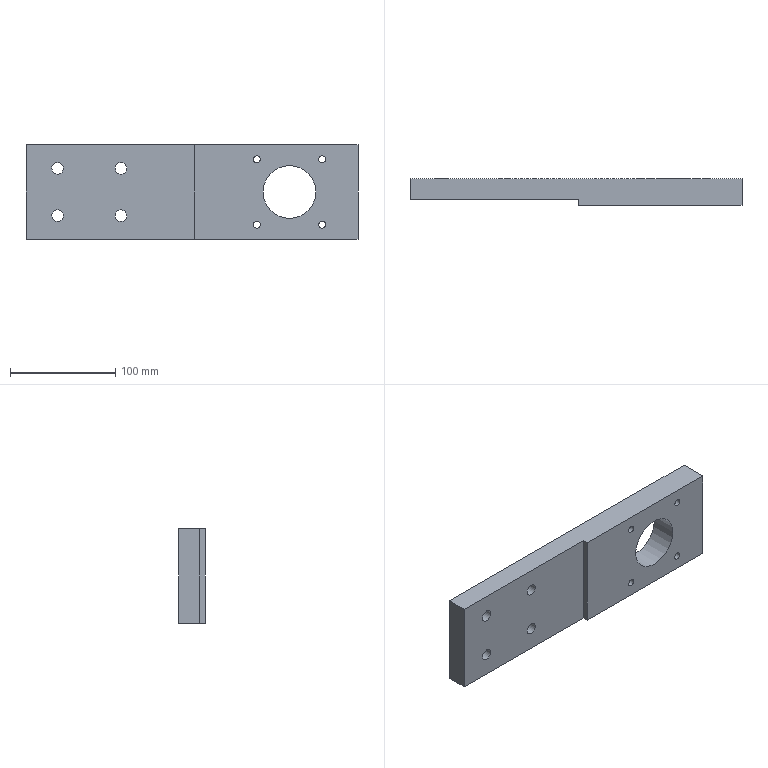Part | STEP file | SN10_002_002_PLACA | 1 solid | 17 faces | box 315 x 25 x 90 mm | volume 576590 mm3 | cylinder 9 | plane 8 | commonest cylinder face diameters 6.647 x4 11 x4 50 x1
STEP:
#1=CARTESIAN_POINT('',(0.,0.,0.));
#2=DIRECTION('',(0.,0.,1.));
#3=DIRECTION('',(1.,0.,0.));
#4=AXIS2_PLACEMENT_3D('',#1,#2,#3);
#5=CARTESIAN_POINT('',(5971.917,200.,32.593));
#6=VERTEX_POINT('',#5);
#7=CARTESIAN_POINT('',(5969.,200.,31.));
#8=DIRECTION('',(0.,-1.,0.));
#9=DIRECTION('',(1.,0.,0.));
#10=AXIS2_PLACEMENT_3D('',#7,#8,#9);
#11=CIRCLE('',#10,3.324);
#12=CARTESIAN_POINT('',(5969.,199.9,31.));
#13=DIRECTION('',(0.,-1.,0.));
#14=DIRECTION('',(0.8776,0.,0.4794));
#15=AXIS2_PLACEMENT_3D('',#12,#13,#14);
#16=CYLINDRICAL_SURFACE('',#15,3.324);
#17=CARTESIAN_POINT('',(-0.5,-0.1));
#18=DIRECTION('',(1.,0.));
#19=VECTOR('',#18,1.);
#20=LINE('',#17,#19);
#21=(GEOMETRIC_REPRESENTATION_CONTEXT(2)PARAMETRIC_REPRESENTATION_CONTEXT()REPRESENTATION_CONTEXT('',''));
#22=DEFINITIONAL_REPRESENTATION('',(#20),#21);
#23=PCURVE('',#16,#22);
#24=CARTESIAN_POINT('',(6065.,200.,45.));
#25=DIRECTION('',(0.,-1.,0.));
#26=DIRECTION('',(0.,0.,-1.));
#27=AXIS2_PLACEMENT_3D('',#24,#25,#26);
#28=PLANE('',#27);
#29=CARTESIAN_POINT('',(14.,-96.));
#30=DIRECTION('',(0.,1.));
#31=AXIS2_PLACEMENT_2D('',#29,#30);
#32=CIRCLE('',#31,3.324);
#33=(GEOMETRIC_REPRESENTATION_CONTEXT(2)PARAMETRIC_REPRESENTATION_CONTEXT()REPRESENTATION_CONTEXT('',''));
#34=DEFINITIONAL_REPRESENTATION('',(#32),#33);
#35=PCURVE('',#28,#34);
#36=SURFACE_CURVE('',#11,(#23,#35),.PCURVE_S1.);
#37=EDGE_CURVE('',#6,#6,#36,.T.);
#38=ORIENTED_EDGE('',*,*,#37,.T.);
#39=CARTESIAN_POINT('',(5971.917,175.,32.593));
#40=VERTEX_POINT('',#39);
#41=CARTESIAN_POINT('',(5971.917,200.,32.593));
#42=CARTESIAN_POINT('',(5971.917,175.,32.593));
#43=B_SPLINE_CURVE_WITH_KNOTS('',1,(#41,#42),.UNSPECIFIED.,.F.,.F.,(2,2),(-0.1,24.9),.PIECEWISE_BEZIER_KNOTS.);
#44=CARTESIAN_POINT('',(6.283,0.));
#45=DIRECTION('',(0.,1.));
#46=VECTOR('',#45,1.);
#47=LINE('',#44,#46);
#48=(GEOMETRIC_REPRESENTATION_CONTEXT(2)PARAMETRIC_REPRESENTATION_CONTEXT()REPRESENTATION_CONTEXT('',''));
#49=DEFINITIONAL_REPRESENTATION('',(#47),#48);
#50=PCURVE('',#16,#49);
#51=CARTESIAN_POINT('',(0.,0.));
#52=DIRECTION('',(0.,1.));
#53=VECTOR('',#52,1.);
#54=LINE('',#51,#53);
#55=(GEOMETRIC_REPRESENTATION_CONTEXT(2)PARAMETRIC_REPRESENTATION_CONTEXT()REPRESENTATION_CONTEXT('',''));
#56=DEFINITIONAL_REPRESENTATION('',(#54),#55);
#57=PCURVE('',#16,#56);
#58=SEAM_CURVE('',#43,(#50,#57),.PCURVE_S1.);
#59=EDGE_CURVE('',#6,#40,#58,.T.);
#60=ORIENTED_EDGE('',*,*,#59,.T.);
#61=CARTESIAN_POINT('',(5969.,175.,31.));
#62=DIRECTION('',(0.,-1.,0.));
#63=DIRECTION('',(1.,0.,0.));
#64=AXIS2_PLACEMENT_3D('',#61,#62,#63);
#65=CIRCLE('',#64,3.324);
#66=CARTESIAN_POINT('',(-0.5,24.9));
#67=DIRECTION('',(1.,0.));
#68=VECTOR('',#67,1.);
#69=LINE('',#66,#68);
#70=(GEOMETRIC_REPRESENTATION_CONTEXT(2)PARAMETRIC_REPRESENTATION_CONTEXT()REPRESENTATION_CONTEXT('',''));
#71=DEFINITIONAL_REPRESENTATION('',(#69),#70);
#72=PCURVE('',#16,#71);
#73=CARTESIAN_POINT('',(5910.,175.,45.));
#74=DIRECTION('',(0.,1.,0.));
#75=DIRECTION('',(0.,0.,1.));
#76=AXIS2_PLACEMENT_3D('',#73,#74,#75);
#77=PLANE('',#76);
#78=CARTESIAN_POINT('',(-14.,62.324));
#79=CARTESIAN_POINT('',(-8.244,62.324));
#80=CARTESIAN_POINT('',(-11.122,57.338));
#81=CARTESIAN_POINT('',(-14.,52.353));
#82=CARTESIAN_POINT('',(-16.878,57.338));
#83=CARTESIAN_POINT('',(-19.756,62.324));
#84=CARTESIAN_POINT('',(-14.,62.324));
#85=(BOUNDED_CURVE()B_SPLINE_CURVE(2,(#78,#79,#80,#81,#82,#83,#84),.UNSPECIFIED.,.T.,.F.)B_SPLINE_CURVE_WITH_KNOTS((1,2,2,2,2,1),(-2.094,0.,2.094,4.189,6.283,8.378),.UNSPECIFIED.)CURVE()GEOMETRIC_REPRESENTATION_ITEM()RATIONAL_B_SPLINE_CURVE((1.,0.5,1.,0.5,1.,0.5,1.))REPRESENTATION_ITEM(''));
#86=(GEOMETRIC_REPRESENTATION_CONTEXT(2)PARAMETRIC_REPRESENTATION_CONTEXT()REPRESENTATION_CONTEXT('',''));
#87=DEFINITIONAL_REPRESENTATION('',(#85),#86);
#88=PCURVE('',#77,#87);
#89=SURFACE_CURVE('',#65,(#72,#88),.PCURVE_S1.);
#90=EDGE_CURVE('',#40,#40,#89,.T.);
#91=ORIENTED_EDGE('',*,*,#90,.F.);
#92=ORIENTED_EDGE('',*,*,#59,.F.);
#93=EDGE_LOOP('',(#38,#60,#91,#92));
#94=FACE_BOUND('',#93,.F.);
#95=ADVANCED_FACE('',(#94),#16,.F.);
#96=CARTESIAN_POINT('',(6065.,175.,-45.));
#97=VERTEX_POINT('',#96);
#98=CARTESIAN_POINT('',(6065.,200.,-45.));
#99=VERTEX_POINT('',#98);
#100=CARTESIAN_POINT('',(6065.,175.,-45.));
#101=DIRECTION('',(0.,1.,0.));
#102=VECTOR('',#101,1.);
#103=LINE('',#100,#102);
#104=CARTESIAN_POINT('',(6065.,175.,45.));
#105=DIRECTION('',(-1.,0.,0.));
#106=DIRECTION('',(0.,0.,1.));
#107=AXIS2_PLACEMENT_3D('',#104,#105,#106);
#108=PLANE('',#107);
#109=CARTESIAN_POINT('',(-90.,0.));
#110=DIRECTION('',(0.,1.));
#111=VECTOR('',#110,1.);
#112=LINE('',#109,#111);
#113=(GEOMETRIC_REPRESENTATION_CONTEXT(2)PARAMETRIC_REPRESENTATION_CONTEXT()REPRESENTATION_CONTEXT('',''));
#114=DEFINITIONAL_REPRESENTATION('',(#112),#113);
#115=PCURVE('',#108,#114);
#116=CARTESIAN_POINT('',(0.,0.,-45.));
#117=DIRECTION('',(0.,0.,1.));
#118=DIRECTION('',(1.,0.,0.));
#119=AXIS2_PLACEMENT_3D('',#116,#117,#118);
#120=PLANE('',#119);
#121=CARTESIAN_POINT('',(6065.,175.));
#122=DIRECTION('',(0.,1.));
#123=VECTOR('',#122,1.);
#124=LINE('',#121,#123);
#125=(GEOMETRIC_REPRESENTATION_CONTEXT(2)PARAMETRIC_REPRESENTATION_CONTEXT()REPRESENTATION_CONTEXT('',''));
#126=DEFINITIONAL_REPRESENTATION('',(#124),#125);
#127=PCURVE('',#120,#126);
#128=SURFACE_CURVE('',#103,(#115,#127),.PCURVE_S1.);
#129=EDGE_CURVE('',#97,#99,#128,.T.);
#130=ORIENTED_EDGE('',*,*,#129,.T.);
#131=CARTESIAN_POINT('',(6065.,200.,45.));
#132=VERTEX_POINT('',#131);
#133=CARTESIAN_POINT('',(6065.,200.,45.));
#134=DIRECTION('',(0.,0.,-1.));
#135=VECTOR('',#134,1.);
#136=LINE('',#133,#135);
#137=CARTESIAN_POINT('',(0.,25.));
#138=DIRECTION('',(-1.,0.));
#139=VECTOR('',#138,1.);
#140=LINE('',#137,#139);
#141=(GEOMETRIC_REPRESENTATION_CONTEXT(2)PARAMETRIC_REPRESENTATION_CONTEXT()REPRESENTATION_CONTEXT('',''));
#142=DEFINITIONAL_REPRESENTATION('',(#140),#141);
#143=PCURVE('',#108,#142);
#144=CARTESIAN_POINT('',(0.,0.));
#145=DIRECTION('',(1.,0.));
#146=VECTOR('',#145,1.);
#147=LINE('',#144,#146);
#148=(GEOMETRIC_REPRESENTATION_CONTEXT(2)PARAMETRIC_REPRESENTATION_CONTEXT()REPRESENTATION_CONTEXT('',''));
#149=DEFINITIONAL_REPRESENTATION('',(#147),#148);
#150=PCURVE('',#28,#149);
#151=SURFACE_CURVE('',#136,(#143,#150),.PCURVE_S1.);
#152=EDGE_CURVE('',#132,#99,#151,.T.);
#153=ORIENTED_EDGE('',*,*,#152,.F.);
#154=CARTESIAN_POINT('',(6065.,175.,45.));
#155=VERTEX_POINT('',#154);
#156=CARTESIAN_POINT('',(6065.,175.,45.));
#157=DIRECTION('',(0.,1.,0.));
#158=VECTOR('',#157,1.);
#159=LINE('',#156,#158);
#160=CARTESIAN_POINT('',(0.,0.));
#161=DIRECTION('',(0.,1.));
#162=VECTOR('',#161,1.);
#163=LINE('',#160,#162);
#164=(GEOMETRIC_REPRESENTATION_CONTEXT(2)PARAMETRIC_REPRESENTATION_CONTEXT()REPRESENTATION_CONTEXT('',''));
#165=DEFINITIONAL_REPRESENTATION('',(#163),#164);
#166=PCURVE('',#108,#165);
#167=CARTESIAN_POINT('',(0.,0.,45.));
#168=DIRECTION('',(0.,0.,1.));
#169=DIRECTION('',(1.,0.,0.));
#170=AXIS2_PLACEMENT_3D('',#167,#168,#169);
#171=PLANE('',#170);
#172=CARTESIAN_POINT('',(6065.,175.));
#173=DIRECTION('',(0.,1.));
#174=VECTOR('',#173,1.);
#175=LINE('',#172,#174);
#176=(GEOMETRIC_REPRESENTATION_CONTEXT(2)PARAMETRIC_REPRESENTATION_CONTEXT()REPRESENTATION_CONTEXT('',''));
#177=DEFINITIONAL_REPRESENTATION('',(#175),#176);
#178=PCURVE('',#171,#177);
#179=SURFACE_CURVE('',#159,(#166,#178),.PCURVE_S1.);
#180=EDGE_CURVE('',#155,#132,#179,.T.);
#181=ORIENTED_EDGE('',*,*,#180,.F.);
#182=CARTESIAN_POINT('',(6065.,175.,45.));
#183=DIRECTION('',(0.,0.,-1.));
#184=VECTOR('',#183,1.);
#185=LINE('',#182,#184);
#186=CARTESIAN_POINT('',(0.,0.));
#187=DIRECTION('',(-1.,0.));
#188=VECTOR('',#187,1.);
#189=LINE('',#186,#188);
#190=(GEOMETRIC_REPRESENTATION_CONTEXT(2)PARAMETRIC_REPRESENTATION_CONTEXT()REPRESENTATION_CONTEXT('',''));
#191=DEFINITIONAL_REPRESENTATION('',(#189),#190);
#192=PCURVE('',#108,#191);
#193=CARTESIAN_POINT('',(0.,155.));
#194=DIRECTION('',(-1.,0.));
#195=VECTOR('',#194,1.);
#196=LINE('',#193,#195);
#197=(GEOMETRIC_REPRESENTATION_CONTEXT(2)PARAMETRIC_REPRESENTATION_CONTEXT()REPRESENTATION_CONTEXT('',''));
#198=DEFINITIONAL_REPRESENTATION('',(#196),#197);
#199=PCURVE('',#77,#198);
#200=SURFACE_CURVE('',#185,(#192,#199),.PCURVE_S1.);
#201=EDGE_CURVE('',#155,#97,#200,.T.);
#202=ORIENTED_EDGE('',*,*,#201,.T.);
#203=EDGE_LOOP('',(#130,#153,#181,#202));
#204=FACE_BOUND('',#203,.T.);
#205=ADVANCED_FACE('',(#204),#108,.F.);
#206=CARTESIAN_POINT('',(5750.,200.,-45.));
#207=VERTEX_POINT('',#206);
#208=CARTESIAN_POINT('',(5750.,180.,-45.));
#209=VERTEX_POINT('',#208);
#210=CARTESIAN_POINT('',(5750.,200.,-45.));
#211=DIRECTION('',(0.,-1.,0.));
#212=VECTOR('',#211,1.);
#213=LINE('',#210,#212);
#214=CARTESIAN_POINT('',(5750.,200.));
#215=DIRECTION('',(0.,-1.));
#216=VECTOR('',#215,1.);
#217=LINE('',#214,#216);
#218=(GEOMETRIC_REPRESENTATION_CONTEXT(2)PARAMETRIC_REPRESENTATION_CONTEXT()REPRESENTATION_CONTEXT('',''));
#219=DEFINITIONAL_REPRESENTATION('',(#217),#218);
#220=PCURVE('',#120,#219);
#221=CARTESIAN_POINT('',(5750.,200.,45.));
#222=DIRECTION('',(1.,0.,0.));
#223=DIRECTION('',(0.,0.,-1.));
#224=AXIS2_PLACEMENT_3D('',#221,#222,#223);
#225=PLANE('',#224);
#226=CARTESIAN_POINT('',(90.,0.));
#227=DIRECTION('',(0.,-1.));
#228=VECTOR('',#227,1.);
#229=LINE('',#226,#228);
#230=(GEOMETRIC_REPRESENTATION_CONTEXT(2)PARAMETRIC_REPRESENTATION_CONTEXT()REPRESENTATION_CONTEXT('',''));
#231=DEFINITIONAL_REPRESENTATION('',(#229),#230);
#232=PCURVE('',#225,#231);
#233=SURFACE_CURVE('',#213,(#220,#232),.PCURVE_S1.);
#234=EDGE_CURVE('',#207,#209,#233,.T.);
#235=ORIENTED_EDGE('',*,*,#234,.F.);
#236=CARTESIAN_POINT('',(6065.,200.,-45.));
#237=DIRECTION('',(-1.,0.,0.));
#238=VECTOR('',#237,1.);
#239=LINE('',#236,#238);
#240=CARTESIAN_POINT('',(6065.,200.));
#241=DIRECTION('',(-1.,0.));
#242=VECTOR('',#241,1.);
#243=LINE('',#240,#242);
#244=(GEOMETRIC_REPRESENTATION_CONTEXT(2)PARAMETRIC_REPRESENTATION_CONTEXT()REPRESENTATION_CONTEXT('',''));
#245=DEFINITIONAL_REPRESENTATION('',(#243),#244);
#246=PCURVE('',#120,#245);
#247=CARTESIAN_POINT('',(90.,0.));
#248=DIRECTION('',(0.,-1.));
#249=VECTOR('',#248,1.);
#250=LINE('',#247,#249);
#251=(GEOMETRIC_REPRESENTATION_CONTEXT(2)PARAMETRIC_REPRESENTATION_CONTEXT()REPRESENTATION_CONTEXT('',''));
#252=DEFINITIONAL_REPRESENTATION('',(#250),#251);
#253=PCURVE('',#28,#252);
#254=SURFACE_CURVE('',#239,(#246,#253),.PCURVE_S1.);
#255=EDGE_CURVE('',#99,#207,#254,.T.);
#256=ORIENTED_EDGE('',*,*,#255,.F.);
#257=ORIENTED_EDGE('',*,*,#129,.F.);
#258=CARTESIAN_POINT('',(5910.,175.,-45.));
#259=VERTEX_POINT('',#258);
#260=CARTESIAN_POINT('',(5910.,175.,-45.));
#261=DIRECTION('',(1.,0.,0.));
#262=VECTOR('',#261,1.);
#263=LINE('',#260,#262);
#264=CARTESIAN_POINT('',(5910.,175.));
#265=DIRECTION('',(1.,0.));
#266=VECTOR('',#265,1.);
#267=LINE('',#264,#266);
#268=(GEOMETRIC_REPRESENTATION_CONTEXT(2)PARAMETRIC_REPRESENTATION_CONTEXT()REPRESENTATION_CONTEXT('',''));
#269=DEFINITIONAL_REPRESENTATION('',(#267),#268);
#270=PCURVE('',#120,#269);
#271=CARTESIAN_POINT('',(-90.,0.));
#272=DIRECTION('',(0.,1.));
#273=VECTOR('',#272,1.);
#274=LINE('',#271,#273);
#275=(GEOMETRIC_REPRESENTATION_CONTEXT(2)PARAMETRIC_REPRESENTATION_CONTEXT()REPRESENTATION_CONTEXT('',''));
#276=DEFINITIONAL_REPRESENTATION('',(#274),#275);
#277=PCURVE('',#77,#276);
#278=SURFACE_CURVE('',#263,(#270,#277),.PCURVE_S1.);
#279=EDGE_CURVE('',#259,#97,#278,.T.);
#280=ORIENTED_EDGE('',*,*,#279,.F.);
#281=CARTESIAN_POINT('',(5910.,180.,-45.));
#282=VERTEX_POINT('',#281);
#283=CARTESIAN_POINT('',(5910.,180.,-45.));
#284=DIRECTION('',(0.,-1.,0.));
#285=VECTOR('',#284,1.);
#286=LINE('',#283,#285);
#287=CARTESIAN_POINT('',(5910.,180.));
#288=DIRECTION('',(0.,-1.));
#289=VECTOR('',#288,1.);
#290=LINE('',#287,#289);
#291=(GEOMETRIC_REPRESENTATION_CONTEXT(2)PARAMETRIC_REPRESENTATION_CONTEXT()REPRESENTATION_CONTEXT('',''));
#292=DEFINITIONAL_REPRESENTATION('',(#290),#291);
#293=PCURVE('',#120,#292);
#294=CARTESIAN_POINT('',(5910.,180.,45.));
#295=DIRECTION('',(1.,0.,0.));
#296=DIRECTION('',(0.,0.,-1.));
#297=AXIS2_PLACEMENT_3D('',#294,#295,#296);
#298=PLANE('',#297);
#299=CARTESIAN_POINT('',(90.,0.));
#300=DIRECTION('',(0.,-1.));
#301=VECTOR('',#300,1.);
#302=LINE('',#299,#301);
#303=(GEOMETRIC_REPRESENTATION_CONTEXT(2)PARAMETRIC_REPRESENTATION_CONTEXT()REPRESENTATION_CONTEXT('',''));
#304=DEFINITIONAL_REPRESENTATION('',(#302),#303);
#305=PCURVE('',#298,#304);
#306=SURFACE_CURVE('',#286,(#293,#305),.PCURVE_S1.);
#307=EDGE_CURVE('',#282,#259,#306,.T.);
#308=ORIENTED_EDGE('',*,*,#307,.F.);
#309=CARTESIAN_POINT('',(5750.,180.,-45.));
#310=DIRECTION('',(1.,0.,0.));
#311=VECTOR('',#310,1.);
#312=LINE('',#309,#311);
#313=CARTESIAN_POINT('',(5750.,180.));
#314=DIRECTION('',(1.,0.));
#315=VECTOR('',#314,1.);
#316=LINE('',#313,#315);
#317=(GEOMETRIC_REPRESENTATION_CONTEXT(2)PARAMETRIC_REPRESENTATION_CONTEXT()REPRESENTATION_CONTEXT('',''));
#318=DEFINITIONAL_REPRESENTATION('',(#316),#317);
#319=PCURVE('',#120,#318);
#320=CARTESIAN_POINT('',(5750.,180.,45.));
#321=DIRECTION('',(0.,1.,0.));
#322=DIRECTION('',(0.,0.,1.));
#323=AXIS2_PLACEMENT_3D('',#320,#321,#322);
#324=PLANE('',#323);
#325=CARTESIAN_POINT('',(-90.,0.));
#326=DIRECTION('',(0.,1.));
#327=VECTOR('',#326,1.);
#328=LINE('',#325,#327);
#329=(GEOMETRIC_REPRESENTATION_CONTEXT(2)PARAMETRIC_REPRESENTATION_CONTEXT()REPRESENTATION_CONTEXT('',''));
#330=DEFINITIONAL_REPRESENTATION('',(#328),#329);
#331=PCURVE('',#324,#330);
#332=SURFACE_CURVE('',#312,(#319,#331),.PCURVE_S1.);
#333=EDGE_CURVE('',#209,#282,#332,.T.);
#334=ORIENTED_EDGE('',*,*,#333,.F.);
#335=EDGE_LOOP('',(#235,#256,#257,#280,#308,#334));
#336=FACE_BOUND('',#335,.T.);
#337=ADVANCED_FACE('',(#336),#120,.F.);
#338=CARTESIAN_POINT('',(5775.173,200.,19.863));
#339=VERTEX_POINT('',#338);
#340=CARTESIAN_POINT('',(5780.,200.,22.5));
#341=DIRECTION('',(0.,-1.,0.));
#342=DIRECTION('',(1.,0.,0.));
#343=AXIS2_PLACEMENT_3D('',#340,#341,#342);
#344=CIRCLE('',#343,5.5);
#345=CARTESIAN_POINT('',(5780.,199.9,22.5));
#346=DIRECTION('',(0.,-1.,0.));
#347=DIRECTION('',(0.8776,0.,0.4794));
#348=AXIS2_PLACEMENT_3D('',#345,#346,#347);
#349=CYLINDRICAL_SURFACE('',#348,5.5);
#350=CARTESIAN_POINT('',(-0.5,-0.1));
#351=DIRECTION('',(1.,0.));
#352=VECTOR('',#351,1.);
#353=LINE('',#350,#352);
#354=(GEOMETRIC_REPRESENTATION_CONTEXT(2)PARAMETRIC_REPRESENTATION_CONTEXT()REPRESENTATION_CONTEXT('',''));
#355=DEFINITIONAL_REPRESENTATION('',(#353),#354);
#356=PCURVE('',#349,#355);
#357=CARTESIAN_POINT('',(22.5,-285.));
#358=DIRECTION('',(0.,1.));
#359=AXIS2_PLACEMENT_2D('',#357,#358);
#360=CIRCLE('',#359,5.5);
#361=(GEOMETRIC_REPRESENTATION_CONTEXT(2)PARAMETRIC_REPRESENTATION_CONTEXT()REPRESENTATION_CONTEXT('',''));
#362=DEFINITIONAL_REPRESENTATION('',(#360),#361);
#363=PCURVE('',#28,#362);
#364=SURFACE_CURVE('',#344,(#356,#363),.PCURVE_S1.);
#365=EDGE_CURVE('',#339,#339,#364,.T.);
#366=ORIENTED_EDGE('',*,*,#365,.T.);
#367=CARTESIAN_POINT('',(5775.173,180.,19.863));
#368=VERTEX_POINT('',#367);
#369=CARTESIAN_POINT('',(5775.173,200.,19.863));
#370=CARTESIAN_POINT('',(5775.173,180.,19.863));
#371=B_SPLINE_CURVE_WITH_KNOTS('',1,(#369,#370),.UNSPECIFIED.,.F.,.F.,(2,2),(-0.1,19.9),.PIECEWISE_BEZIER_KNOTS.);
#372=CARTESIAN_POINT('',(9.425,0.));
#373=DIRECTION('',(0.,1.));
#374=VECTOR('',#373,1.);
#375=LINE('',#372,#374);
#376=(GEOMETRIC_REPRESENTATION_CONTEXT(2)PARAMETRIC_REPRESENTATION_CONTEXT()REPRESENTATION_CONTEXT('',''));
#377=DEFINITIONAL_REPRESENTATION('',(#375),#376);
#378=PCURVE('',#349,#377);
#379=CARTESIAN_POINT('',(3.142,0.));
#380=DIRECTION('',(0.,1.));
#381=VECTOR('',#380,1.);
#382=LINE('',#379,#381);
#383=(GEOMETRIC_REPRESENTATION_CONTEXT(2)PARAMETRIC_REPRESENTATION_CONTEXT()REPRESENTATION_CONTEXT('',''));
#384=DEFINITIONAL_REPRESENTATION('',(#382),#383);
#385=PCURVE('',#349,#384);
#386=SEAM_CURVE('',#371,(#378,#385),.PCURVE_S1.);
#387=EDGE_CURVE('',#339,#368,#386,.T.);
#388=ORIENTED_EDGE('',*,*,#387,.T.);
#389=CARTESIAN_POINT('',(5780.,180.,22.5));
#390=DIRECTION('',(0.,-1.,0.));
#391=DIRECTION('',(1.,0.,0.));
#392=AXIS2_PLACEMENT_3D('',#389,#390,#391);
#393=CIRCLE('',#392,5.5);
#394=CARTESIAN_POINT('',(-0.5,19.9));
#395=DIRECTION('',(1.,0.));
#396=VECTOR('',#395,1.);
#397=LINE('',#394,#396);
#398=(GEOMETRIC_REPRESENTATION_CONTEXT(2)PARAMETRIC_REPRESENTATION_CONTEXT()REPRESENTATION_CONTEXT('',''));
#399=DEFINITIONAL_REPRESENTATION('',(#397),#398);
#400=PCURVE('',#349,#399);
#401=CARTESIAN_POINT('',(-22.5,35.5));
#402=CARTESIAN_POINT('',(-12.974,35.5));
#403=CARTESIAN_POINT('',(-17.737,27.25));
#404=CARTESIAN_POINT('',(-22.5,19.));
#405=CARTESIAN_POINT('',(-27.263,27.25));
#406=CARTESIAN_POINT('',(-32.026,35.5));
#407=CARTESIAN_POINT('',(-22.5,35.5));
#408=(BOUNDED_CURVE()B_SPLINE_CURVE(2,(#401,#402,#403,#404,#405,#406,#407),.UNSPECIFIED.,.T.,.F.)B_SPLINE_CURVE_WITH_KNOTS((1,2,2,2,2,1),(-2.094,0.,2.094,4.189,6.283,8.378),.UNSPECIFIED.)CURVE()GEOMETRIC_REPRESENTATION_ITEM()RATIONAL_B_SPLINE_CURVE((1.,0.5,1.,0.5,1.,0.5,1.))REPRESENTATION_ITEM(''));
#409=(GEOMETRIC_REPRESENTATION_CONTEXT(2)PARAMETRIC_REPRESENTATION_CONTEXT()REPRESENTATION_CONTEXT('',''));
#410=DEFINITIONAL_REPRESENTATION('',(#408),#409);
#411=PCURVE('',#324,#410);
#412=SURFACE_CURVE('',#393,(#400,#411),.PCURVE_S1.);
#413=EDGE_CURVE('',#368,#368,#412,.T.);
#414=ORIENTED_EDGE('',*,*,#413,.F.);
#415=ORIENTED_EDGE('',*,*,#387,.F.);
#416=EDGE_LOOP('',(#366,#388,#414,#415));
#417=FACE_BOUND('',#416,.F.);
#418=ADVANCED_FACE('',(#417),#349,.F.);
#419=CARTESIAN_POINT('',(5975.,200.,0.));
#420=VERTEX_POINT('',#419);
#421=CARTESIAN_POINT('',(6000.,200.,0.));
#422=DIRECTION('',(0.,-1.,0.));
#423=DIRECTION('',(1.,0.,0.));
#424=AXIS2_PLACEMENT_3D('',#421,#422,#423);
#425=CIRCLE('',#424,25.);
#426=CARTESIAN_POINT('',(6000.,188.16,0.));
#427=DIRECTION('',(0.,-1.,0.));
#428=DIRECTION('',(1.,0.,0.));
#429=AXIS2_PLACEMENT_3D('',#426,#427,#428);
#430=CYLINDRICAL_SURFACE('',#429,25.);
#431=CARTESIAN_POINT('',(0.,-11.84));
#432=DIRECTION('',(1.,0.));
#433=VECTOR('',#432,1.);
#434=LINE('',#431,#433);
#435=(GEOMETRIC_REPRESENTATION_CONTEXT(2)PARAMETRIC_REPRESENTATION_CONTEXT()REPRESENTATION_CONTEXT('',''));
#436=DEFINITIONAL_REPRESENTATION('',(#434),#435);
#437=PCURVE('',#430,#436);
#438=CARTESIAN_POINT('',(45.,-65.));
#439=DIRECTION('',(0.,1.));
#440=AXIS2_PLACEMENT_2D('',#438,#439);
#441=CIRCLE('',#440,25.);
#442=(GEOMETRIC_REPRESENTATION_CONTEXT(2)PARAMETRIC_REPRESENTATION_CONTEXT()REPRESENTATION_CONTEXT('',''));
#443=DEFINITIONAL_REPRESENTATION('',(#441),#442);
#444=PCURVE('',#28,#443);
#445=SURFACE_CURVE('',#425,(#437,#444),.PCURVE_S1.);
#446=EDGE_CURVE('',#420,#420,#445,.T.);
#447=ORIENTED_EDGE('',*,*,#446,.T.);
#448=CARTESIAN_POINT('',(5975.,175.,0.));
#449=VERTEX_POINT('',#448);
#450=CARTESIAN_POINT('',(5975.,200.,0.));
#451=CARTESIAN_POINT('',(5975.,175.,0.));
#452=B_SPLINE_CURVE_WITH_KNOTS('',1,(#450,#451),.UNSPECIFIED.,.F.,.F.,(2,2),(-11.84,13.16),.PIECEWISE_BEZIER_KNOTS.);
#453=CARTESIAN_POINT('',(9.425,0.));
#454=DIRECTION('',(0.,1.));
#455=VECTOR('',#454,1.);
#456=LINE('',#453,#455);
#457=(GEOMETRIC_REPRESENTATION_CONTEXT(2)PARAMETRIC_REPRESENTATION_CONTEXT()REPRESENTATION_CONTEXT('',''));
#458=DEFINITIONAL_REPRESENTATION('',(#456),#457);
#459=PCURVE('',#430,#458);
#460=CARTESIAN_POINT('',(3.142,0.));
#461=DIRECTION('',(0.,1.));
#462=VECTOR('',#461,1.);
#463=LINE('',#460,#462);
#464=(GEOMETRIC_REPRESENTATION_CONTEXT(2)PARAMETRIC_REPRESENTATION_CONTEXT()REPRESENTATION_CONTEXT('',''));
#465=DEFINITIONAL_REPRESENTATION('',(#463),#464);
#466=PCURVE('',#430,#465);
#467=SEAM_CURVE('',#452,(#459,#466),.PCURVE_S1.);
#468=EDGE_CURVE('',#420,#449,#467,.T.);
#469=ORIENTED_EDGE('',*,*,#468,.T.);
#470=CARTESIAN_POINT('',(6000.,175.,0.));
#471=DIRECTION('',(0.,-1.,0.));
#472=DIRECTION('',(1.,0.,0.));
#473=AXIS2_PLACEMENT_3D('',#470,#471,#472);
#474=CIRCLE('',#473,25.);
#475=CARTESIAN_POINT('',(0.,13.16));
#476=DIRECTION('',(1.,0.));
#477=VECTOR('',#476,1.);
#478=LINE('',#475,#477);
#479=(GEOMETRIC_REPRESENTATION_CONTEXT(2)PARAMETRIC_REPRESENTATION_CONTEXT()REPRESENTATION_CONTEXT('',''));
#480=DEFINITIONAL_REPRESENTATION('',(#478),#479);
#481=PCURVE('',#430,#480);
#482=CARTESIAN_POINT('',(-45.,115.));
#483=CARTESIAN_POINT('',(-1.699,115.));
#484=CARTESIAN_POINT('',(-23.349,77.5));
#485=CARTESIAN_POINT('',(-45.,40.));
#486=CARTESIAN_POINT('',(-66.651,77.5));
#487=CARTESIAN_POINT('',(-88.301,115.));
#488=CARTESIAN_POINT('',(-45.,115.));
#489=(BOUNDED_CURVE()B_SPLINE_CURVE(2,(#482,#483,#484,#485,#486,#487,#488),.UNSPECIFIED.,.T.,.F.)B_SPLINE_CURVE_WITH_KNOTS((1,2,2,2,2,1),(-2.094,0.,2.094,4.189,6.283,8.378),.UNSPECIFIED.)CURVE()GEOMETRIC_REPRESENTATION_ITEM()RATIONAL_B_SPLINE_CURVE((1.,0.5,1.,0.5,1.,0.5,1.))REPRESENTATION_ITEM(''));
#490=(GEOMETRIC_REPRESENTATION_CONTEXT(2)PARAMETRIC_REPRESENTATION_CONTEXT()REPRESENTATION_CONTEXT('',''));
#491=DEFINITIONAL_REPRESENTATION('',(#489),#490);
#492=PCURVE('',#77,#491);
#493=SURFACE_CURVE('',#474,(#481,#492),.PCURVE_S1.);
#494=EDGE_CURVE('',#449,#449,#493,.T.);
#495=ORIENTED_EDGE('',*,*,#494,.F.);
#496=ORIENTED_EDGE('',*,*,#468,.F.);
#497=EDGE_LOOP('',(#447,#469,#495,#496));
#498=FACE_BOUND('',#497,.F.);
#499=ADVANCED_FACE('',(#498),#430,.F.);
#500=CARTESIAN_POINT('',(5844.827,200.,25.137));
#501=VERTEX_POINT('',#500);
#502=CARTESIAN_POINT('',(5840.,200.,22.5));
#503=DIRECTION('',(0.,-1.,0.));
#504=DIRECTION('',(1.,0.,0.));
#505=AXIS2_PLACEMENT_3D('',#502,#503,#504);
#506=CIRCLE('',#505,5.5);
#507=CARTESIAN_POINT('',(5840.,199.9,22.5));
#508=DIRECTION('',(0.,-1.,0.));
#509=DIRECTION('',(0.8776,0.,0.4794));
#510=AXIS2_PLACEMENT_3D('',#507,#508,#509);
#511=CYLINDRICAL_SURFACE('',#510,5.5);
#512=CARTESIAN_POINT('',(-0.5,-0.1));
#513=DIRECTION('',(1.,0.));
#514=VECTOR('',#513,1.);
#515=LINE('',#512,#514);
#516=(GEOMETRIC_REPRESENTATION_CONTEXT(2)PARAMETRIC_REPRESENTATION_CONTEXT()REPRESENTATION_CONTEXT('',''));
#517=DEFINITIONAL_REPRESENTATION('',(#515),#516);
#518=PCURVE('',#511,#517);
#519=CARTESIAN_POINT('',(22.5,-225.));
#520=DIRECTION('',(0.,1.));
#521=AXIS2_PLACEMENT_2D('',#519,#520);
#522=CIRCLE('',#521,5.5);
#523=(GEOMETRIC_REPRESENTATION_CONTEXT(2)PARAMETRIC_REPRESENTATION_CONTEXT()REPRESENTATION_CONTEXT('',''));
#524=DEFINITIONAL_REPRESENTATION('',(#522),#523);
#525=PCURVE('',#28,#524);
#526=SURFACE_CURVE('',#506,(#518,#525),.PCURVE_S1.);
#527=EDGE_CURVE('',#501,#501,#526,.T.);
#528=ORIENTED_EDGE('',*,*,#527,.T.);
#529=CARTESIAN_POINT('',(5844.827,180.,25.137));
#530=VERTEX_POINT('',#529);
#531=CARTESIAN_POINT('',(5844.827,200.,25.137));
#532=CARTESIAN_POINT('',(5844.827,180.,25.137));
#533=B_SPLINE_CURVE_WITH_KNOTS('',1,(#531,#532),.UNSPECIFIED.,.F.,.F.,(2,2),(-0.1,19.9),.PIECEWISE_BEZIER_KNOTS.);
#534=CARTESIAN_POINT('',(6.283,0.));
#535=DIRECTION('',(0.,1.));
#536=VECTOR('',#535,1.);
#537=LINE('',#534,#536);
#538=(GEOMETRIC_REPRESENTATION_CONTEXT(2)PARAMETRIC_REPRESENTATION_CONTEXT()REPRESENTATION_CONTEXT('',''));
#539=DEFINITIONAL_REPRESENTATION('',(#537),#538);
#540=PCURVE('',#511,#539);
#541=CARTESIAN_POINT('',(0.,0.));
#542=DIRECTION('',(0.,1.));
#543=VECTOR('',#542,1.);
#544=LINE('',#541,#543);
#545=(GEOMETRIC_REPRESENTATION_CONTEXT(2)PARAMETRIC_REPRESENTATION_CONTEXT()REPRESENTATION_CONTEXT('',''));
#546=DEFINITIONAL_REPRESENTATION('',(#544),#545);
#547=PCURVE('',#511,#546);
#548=SEAM_CURVE('',#533,(#540,#547),.PCURVE_S1.);
#549=EDGE_CURVE('',#501,#530,#548,.T.);
#550=ORIENTED_EDGE('',*,*,#549,.T.);
#551=CARTESIAN_POINT('',(5840.,180.,22.5));
#552=DIRECTION('',(0.,-1.,0.));
#553=DIRECTION('',(1.,0.,0.));
#554=AXIS2_PLACEMENT_3D('',#551,#552,#553);
#555=CIRCLE('',#554,5.5);
#556=CARTESIAN_POINT('',(-0.5,19.9));
#557=DIRECTION('',(1.,0.));
#558=VECTOR('',#557,1.);
#559=LINE('',#556,#558);
#560=(GEOMETRIC_REPRESENTATION_CONTEXT(2)PARAMETRIC_REPRESENTATION_CONTEXT()REPRESENTATION_CONTEXT('',''));
#561=DEFINITIONAL_REPRESENTATION('',(#559),#560);
#562=PCURVE('',#511,#561);
#563=CARTESIAN_POINT('',(-22.5,95.5));
#564=CARTESIAN_POINT('',(-12.974,95.5));
#565=CARTESIAN_POINT('',(-17.737,87.25));
#566=CARTESIAN_POINT('',(-22.5,79.));
#567=CARTESIAN_POINT('',(-27.263,87.25));
#568=CARTESIAN_POINT('',(-32.026,95.5));
#569=CARTESIAN_POINT('',(-22.5,95.5));
#570=(BOUNDED_CURVE()B_SPLINE_CURVE(2,(#563,#564,#565,#566,#567,#568,#569),.UNSPECIFIED.,.T.,.F.)B_SPLINE_CURVE_WITH_KNOTS((1,2,2,2,2,1),(-2.094,0.,2.094,4.189,6.283,8.378),.UNSPECIFIED.)CURVE()GEOMETRIC_REPRESENTATION_ITEM()RATIONAL_B_SPLINE_CURVE((1.,0.5,1.,0.5,1.,0.5,1.))REPRESENTATION_ITEM(''));
#571=(GEOMETRIC_REPRESENTATION_CONTEXT(2)PARAMETRIC_REPRESENTATION_CONTEXT()REPRESENTATION_CONTEXT('',''));
#572=DEFINITIONAL_REPRESENTATION('',(#570),#571);
#573=PCURVE('',#324,#572);
#574=SURFACE_CURVE('',#555,(#562,#573),.PCURVE_S1.);
#575=EDGE_CURVE('',#530,#530,#574,.T.);
#576=ORIENTED_EDGE('',*,*,#575,.F.);
#577=ORIENTED_EDGE('',*,*,#549,.F.);
#578=EDGE_LOOP('',(#528,#550,#576,#577));
#579=FACE_BOUND('',#578,.F.);
#580=ADVANCED_FACE('',(#579),#511,.F.);
#581=CARTESIAN_POINT('',(5784.827,200.,-19.863));
#582=VERTEX_POINT('',#581);
#583=CARTESIAN_POINT('',(5780.,200.,-22.5));
#584=DIRECTION('',(0.,-1.,0.));
#585=DIRECTION('',(1.,0.,0.));
#586=AXIS2_PLACEMENT_3D('',#583,#584,#585);
#587=CIRCLE('',#586,5.5);
#588=CARTESIAN_POINT('',(5780.,199.9,-22.5));
#589=DIRECTION('',(0.,-1.,0.));
#590=DIRECTION('',(0.8776,0.,0.4794));
#591=AXIS2_PLACEMENT_3D('',#588,#589,#590);
#592=CYLINDRICAL_SURFACE('',#591,5.5);
#593=CARTESIAN_POINT('',(-0.5,-0.1));
#594=DIRECTION('',(1.,0.));
#595=VECTOR('',#594,1.);
#596=LINE('',#593,#595);
#597=(GEOMETRIC_REPRESENTATION_CONTEXT(2)PARAMETRIC_REPRESENTATION_CONTEXT()REPRESENTATION_CONTEXT('',''));
#598=DEFINITIONAL_REPRESENTATION('',(#596),#597);
#599=PCURVE('',#592,#598);
#600=CARTESIAN_POINT('',(67.5,-285.));
#601=DIRECTION('',(0.,1.));
#602=AXIS2_PLACEMENT_2D('',#600,#601);
#603=CIRCLE('',#602,5.5);
#604=(GEOMETRIC_REPRESENTATION_CONTEXT(2)PARAMETRIC_REPRESENTATION_CONTEXT()REPRESENTATION_CONTEXT('',''));
#605=DEFINITIONAL_REPRESENTATION('',(#603),#604);
#606=PCURVE('',#28,#605);
#607=SURFACE_CURVE('',#587,(#599,#606),.PCURVE_S1.);
#608=EDGE_CURVE('',#582,#582,#607,.T.);
#609=ORIENTED_EDGE('',*,*,#608,.T.);
#610=CARTESIAN_POINT('',(5784.827,180.,-19.863));
#611=VERTEX_POINT('',#610);
#612=CARTESIAN_POINT('',(5784.827,200.,-19.863));
#613=CARTESIAN_POINT('',(5784.827,180.,-19.863));
#614=B_SPLINE_CURVE_WITH_KNOTS('',1,(#612,#613),.UNSPECIFIED.,.F.,.F.,(2,2),(-0.1,19.9),.PIECEWISE_BEZIER_KNOTS.);
#615=CARTESIAN_POINT('',(6.283,0.));
#616=DIRECTION('',(0.,1.));
#617=VECTOR('',#616,1.);
#618=LINE('',#615,#617);
#619=(GEOMETRIC_REPRESENTATION_CONTEXT(2)PARAMETRIC_REPRESENTATION_CONTEXT()REPRESENTATION_CONTEXT('',''));
#620=DEFINITIONAL_REPRESENTATION('',(#618),#619);
#621=PCURVE('',#592,#620);
#622=CARTESIAN_POINT('',(0.,0.));
#623=DIRECTION('',(0.,1.));
#624=VECTOR('',#623,1.);
#625=LINE('',#622,#624);
#626=(GEOMETRIC_REPRESENTATION_CONTEXT(2)PARAMETRIC_REPRESENTATION_CONTEXT()REPRESENTATION_CONTEXT('',''));
#627=DEFINITIONAL_REPRESENTATION('',(#625),#626);
#628=PCURVE('',#592,#627);
#629=SEAM_CURVE('',#614,(#621,#628),.PCURVE_S1.);
#630=EDGE_CURVE('',#582,#611,#629,.T.);
#631=ORIENTED_EDGE('',*,*,#630,.T.);
#632=CARTESIAN_POINT('',(5780.,180.,-22.5));
#633=DIRECTION('',(0.,-1.,0.));
#634=DIRECTION('',(1.,0.,0.));
#635=AXIS2_PLACEMENT_3D('',#632,#633,#634);
#636=CIRCLE('',#635,5.5);
#637=CARTESIAN_POINT('',(-0.5,19.9));
#638=DIRECTION('',(1.,0.));
#639=VECTOR('',#638,1.);
#640=LINE('',#637,#639);
#641=(GEOMETRIC_REPRESENTATION_CONTEXT(2)PARAMETRIC_REPRESENTATION_CONTEXT()REPRESENTATION_CONTEXT('',''));
#642=DEFINITIONAL_REPRESENTATION('',(#640),#641);
#643=PCURVE('',#592,#642);
#644=CARTESIAN_POINT('',(-67.5,35.5));
#645=CARTESIAN_POINT('',(-57.974,35.5));
#646=CARTESIAN_POINT('',(-62.737,27.25));
#647=CARTESIAN_POINT('',(-67.5,19.));
#648=CARTESIAN_POINT('',(-72.263,27.25));
#649=CARTESIAN_POINT('',(-77.026,35.5));
#650=CARTESIAN_POINT('',(-67.5,35.5));
#651=(BOUNDED_CURVE()B_SPLINE_CURVE(2,(#644,#645,#646,#647,#648,#649,#650),.UNSPECIFIED.,.T.,.F.)B_SPLINE_CURVE_WITH_KNOTS((1,2,2,2,2,1),(-2.094,0.,2.094,4.189,6.283,8.378),.UNSPECIFIED.)CURVE()GEOMETRIC_REPRESENTATION_ITEM()RATIONAL_B_SPLINE_CURVE((1.,0.5,1.,0.5,1.,0.5,1.))REPRESENTATION_ITEM(''));
#652=(GEOMETRIC_REPRESENTATION_CONTEXT(2)PARAMETRIC_REPRESENTATION_CONTEXT()REPRESENTATION_CONTEXT('',''));
#653=DEFINITIONAL_REPRESENTATION('',(#651),#652);
#654=PCURVE('',#324,#653);
#655=SURFACE_CURVE('',#636,(#643,#654),.PCURVE_S1.);
#656=EDGE_CURVE('',#611,#611,#655,.T.);
#657=ORIENTED_EDGE('',*,*,#656,.F.);
#658=ORIENTED_EDGE('',*,*,#630,.F.);
#659=EDGE_LOOP('',(#609,#631,#657,#658));
#660=FACE_BOUND('',#659,.F.);
#661=ADVANCED_FACE('',(#660),#592,.F.);
#662=CARTESIAN_POINT('',(5844.827,200.,-19.863));
#663=VERTEX_POINT('',#662);
#664=CARTESIAN_POINT('',(5840.,200.,-22.5));
#665=DIRECTION('',(0.,-1.,0.));
#666=DIRECTION('',(1.,0.,0.));
#667=AXIS2_PLACEMENT_3D('',#664,#665,#666);
#668=CIRCLE('',#667,5.5);
#669=CARTESIAN_POINT('',(5840.,199.9,-22.5));
#670=DIRECTION('',(0.,-1.,0.));
#671=DIRECTION('',(0.8776,0.,0.4794));
#672=AXIS2_PLACEMENT_3D('',#669,#670,#671);
#673=CYLINDRICAL_SURFACE('',#672,5.5);
#674=CARTESIAN_POINT('',(-0.5,-0.1));
#675=DIRECTION('',(1.,0.));
#676=VECTOR('',#675,1.);
#677=LINE('',#674,#676);
#678=(GEOMETRIC_REPRESENTATION_CONTEXT(2)PARAMETRIC_REPRESENTATION_CONTEXT()REPRESENTATION_CONTEXT('',''));
#679=DEFINITIONAL_REPRESENTATION('',(#677),#678);
#680=PCURVE('',#673,#679);
#681=CARTESIAN_POINT('',(67.5,-225.));
#682=DIRECTION('',(0.,1.));
#683=AXIS2_PLACEMENT_2D('',#681,#682);
#684=CIRCLE('',#683,5.5);
#685=(GEOMETRIC_REPRESENTATION_CONTEXT(2)PARAMETRIC_REPRESENTATION_CONTEXT()REPRESENTATION_CONTEXT('',''));
#686=DEFINITIONAL_REPRESENTATION('',(#684),#685);
#687=PCURVE('',#28,#686);
#688=SURFACE_CURVE('',#668,(#680,#687),.PCURVE_S1.);
#689=EDGE_CURVE('',#663,#663,#688,.T.);
#690=ORIENTED_EDGE('',*,*,#689,.T.);
#691=CARTESIAN_POINT('',(5844.827,180.,-19.863));
#692=VERTEX_POINT('',#691);
#693=CARTESIAN_POINT('',(5844.827,200.,-19.863));
#694=CARTESIAN_POINT('',(5844.827,180.,-19.863));
#695=B_SPLINE_CURVE_WITH_KNOTS('',1,(#693,#694),.UNSPECIFIED.,.F.,.F.,(2,2),(-0.1,19.9),.PIECEWISE_BEZIER_KNOTS.);
#696=CARTESIAN_POINT('',(6.283,0.));
#697=DIRECTION('',(0.,1.));
#698=VECTOR('',#697,1.);
#699=LINE('',#696,#698);
#700=(GEOMETRIC_REPRESENTATION_CONTEXT(2)PARAMETRIC_REPRESENTATION_CONTEXT()REPRESENTATION_CONTEXT('',''));
#701=DEFINITIONAL_REPRESENTATION('',(#699),#700);
#702=PCURVE('',#673,#701);
#703=CARTESIAN_POINT('',(0.,0.));
#704=DIRECTION('',(0.,1.));
#705=VECTOR('',#704,1.);
#706=LINE('',#703,#705);
#707=(GEOMETRIC_REPRESENTATION_CONTEXT(2)PARAMETRIC_REPRESENTATION_CONTEXT()REPRESENTATION_CONTEXT('',''));
#708=DEFINITIONAL_REPRESENTATION('',(#706),#707);
#709=PCURVE('',#673,#708);
#710=SEAM_CURVE('',#695,(#702,#709),.PCURVE_S1.);
#711=EDGE_CURVE('',#663,#692,#710,.T.);
#712=ORIENTED_EDGE('',*,*,#711,.T.);
#713=CARTESIAN_POINT('',(5840.,180.,-22.5));
#714=DIRECTION('',(0.,-1.,0.));
#715=DIRECTION('',(1.,0.,0.));
#716=AXIS2_PLACEMENT_3D('',#713,#714,#715);
#717=CIRCLE('',#716,5.5);
#718=CARTESIAN_POINT('',(-0.5,19.9));
#719=DIRECTION('',(1.,0.));
#720=VECTOR('',#719,1.);
#721=LINE('',#718,#720);
#722=(GEOMETRIC_REPRESENTATION_CONTEXT(2)PARAMETRIC_REPRESENTATION_CONTEXT()REPRESENTATION_CONTEXT('',''));
#723=DEFINITIONAL_REPRESENTATION('',(#721),#722);
#724=PCURVE('',#673,#723);
#725=CARTESIAN_POINT('',(-67.5,95.5));
#726=CARTESIAN_POINT('',(-57.974,95.5));
#727=CARTESIAN_POINT('',(-62.737,87.25));
#728=CARTESIAN_POINT('',(-67.5,79.));
#729=CARTESIAN_POINT('',(-72.263,87.25));
#730=CARTESIAN_POINT('',(-77.026,95.5));
#731=CARTESIAN_POINT('',(-67.5,95.5));
#732=(BOUNDED_CURVE()B_SPLINE_CURVE(2,(#725,#726,#727,#728,#729,#730,#731),.UNSPECIFIED.,.T.,.F.)B_SPLINE_CURVE_WITH_KNOTS((1,2,2,2,2,1),(-2.094,0.,2.094,4.189,6.283,8.378),.UNSPECIFIED.)CURVE()GEOMETRIC_REPRESENTATION_ITEM()RATIONAL_B_SPLINE_CURVE((1.,0.5,1.,0.5,1.,0.5,1.))REPRESENTATION_ITEM(''));
#733=(GEOMETRIC_REPRESENTATION_CONTEXT(2)PARAMETRIC_REPRESENTATION_CONTEXT()REPRESENTATION_CONTEXT('',''));
#734=DEFINITIONAL_REPRESENTATION('',(#732),#733);
#735=PCURVE('',#324,#734);
#736=SURFACE_CURVE('',#717,(#724,#735),.PCURVE_S1.);
#737=EDGE_CURVE('',#692,#692,#736,.T.);
#738=ORIENTED_EDGE('',*,*,#737,.F.);
#739=ORIENTED_EDGE('',*,*,#711,.F.);
#740=EDGE_LOOP('',(#690,#712,#738,#739));
#741=FACE_BOUND('',#740,.F.);
#742=ADVANCED_FACE('',(#741),#673,.F.);
#743=ORIENTED_EDGE('',*,*,#307,.T.);
#744=CARTESIAN_POINT('',(5910.,175.,45.));
#745=VERTEX_POINT('',#744);
#746=CARTESIAN_POINT('',(5910.,175.,45.));
#747=DIRECTION('',(0.,0.,-1.));
#748=VECTOR('',#747,1.);
#749=LINE('',#746,#748);
#750=CARTESIAN_POINT('',(0.,-5.));
#751=DIRECTION('',(1.,0.));
#752=VECTOR('',#751,1.);
#753=LINE('',#750,#752);
#754=(GEOMETRIC_REPRESENTATION_CONTEXT(2)PARAMETRIC_REPRESENTATION_CONTEXT()REPRESENTATION_CONTEXT('',''));
#755=DEFINITIONAL_REPRESENTATION('',(#753),#754);
#756=PCURVE('',#298,#755);
#757=CARTESIAN_POINT('',(0.,0.));
#758=DIRECTION('',(-1.,0.));
#759=VECTOR('',#758,1.);
#760=LINE('',#757,#759);
#761=(GEOMETRIC_REPRESENTATION_CONTEXT(2)PARAMETRIC_REPRESENTATION_CONTEXT()REPRESENTATION_CONTEXT('',''));
#762=DEFINITIONAL_REPRESENTATION('',(#760),#761);
#763=PCURVE('',#77,#762);
#764=SURFACE_CURVE('',#749,(#756,#763),.PCURVE_S1.);
#765=EDGE_CURVE('',#745,#259,#764,.T.);
#766=ORIENTED_EDGE('',*,*,#765,.F.);
#767=CARTESIAN_POINT('',(5910.,180.,45.));
#768=VERTEX_POINT('',#767);
#769=CARTESIAN_POINT('',(5910.,180.,45.));
#770=DIRECTION('',(0.,-1.,0.));
#771=VECTOR('',#770,1.);
#772=LINE('',#769,#771);
#773=CARTESIAN_POINT('',(0.,0.));
#774=DIRECTION('',(0.,-1.));
#775=VECTOR('',#774,1.);
#776=LINE('',#773,#775);
#777=(GEOMETRIC_REPRESENTATION_CONTEXT(2)PARAMETRIC_REPRESENTATION_CONTEXT()REPRESENTATION_CONTEXT('',''));
#778=DEFINITIONAL_REPRESENTATION('',(#776),#777);
#779=PCURVE('',#298,#778);
#780=CARTESIAN_POINT('',(5910.,180.));
#781=DIRECTION('',(0.,-1.));
#782=VECTOR('',#781,1.);
#783=LINE('',#780,#782);
#784=(GEOMETRIC_REPRESENTATION_CONTEXT(2)PARAMETRIC_REPRESENTATION_CONTEXT()REPRESENTATION_CONTEXT('',''));
#785=DEFINITIONAL_REPRESENTATION('',(#783),#784);
#786=PCURVE('',#171,#785);
#787=SURFACE_CURVE('',#772,(#779,#786),.PCURVE_S1.);
#788=EDGE_CURVE('',#768,#745,#787,.T.);
#789=ORIENTED_EDGE('',*,*,#788,.F.);
#790=CARTESIAN_POINT('',(5910.,180.,45.));
#791=DIRECTION('',(0.,0.,-1.));
#792=VECTOR('',#791,1.);
#793=LINE('',#790,#792);
#794=CARTESIAN_POINT('',(0.,0.));
#795=DIRECTION('',(1.,0.));
#796=VECTOR('',#795,1.);
#797=LINE('',#794,#796);
#798=(GEOMETRIC_REPRESENTATION_CONTEXT(2)PARAMETRIC_REPRESENTATION_CONTEXT()REPRESENTATION_CONTEXT('',''));
#799=DEFINITIONAL_REPRESENTATION('',(#797),#798);
#800=PCURVE('',#298,#799);
#801=CARTESIAN_POINT('',(0.,160.));
#802=DIRECTION('',(-1.,0.));
#803=VECTOR('',#802,1.);
#804=LINE('',#801,#803);
#805=(GEOMETRIC_REPRESENTATION_CONTEXT(2)PARAMETRIC_REPRESENTATION_CONTEXT()REPRESENTATION_CONTEXT('',''));
#806=DEFINITIONAL_REPRESENTATION('',(#804),#805);
#807=PCURVE('',#324,#806);
#808=SURFACE_CURVE('',#793,(#800,#807),.PCURVE_S1.);
#809=EDGE_CURVE('',#768,#282,#808,.T.);
#810=ORIENTED_EDGE('',*,*,#809,.T.);
#811=EDGE_LOOP('',(#743,#766,#789,#810));
#812=FACE_BOUND('',#811,.T.);
#813=ADVANCED_FACE('',(#812),#298,.F.);
#814=ORIENTED_EDGE('',*,*,#333,.T.);
#815=ORIENTED_EDGE('',*,*,#809,.F.);
#816=CARTESIAN_POINT('',(5750.,180.,45.));
#817=VERTEX_POINT('',#816);
#818=CARTESIAN_POINT('',(5750.,180.,45.));
#819=DIRECTION('',(1.,0.,0.));
#820=VECTOR('',#819,1.);
#821=LINE('',#818,#820);
#822=CARTESIAN_POINT('',(0.,0.));
#823=DIRECTION('',(0.,1.));
#824=VECTOR('',#823,1.);
#825=LINE('',#822,#824);
#826=(GEOMETRIC_REPRESENTATION_CONTEXT(2)PARAMETRIC_REPRESENTATION_CONTEXT()REPRESENTATION_CONTEXT('',''));
#827=DEFINITIONAL_REPRESENTATION('',(#825),#826);
#828=PCURVE('',#324,#827);
#829=CARTESIAN_POINT('',(5750.,180.));
#830=DIRECTION('',(1.,0.));
#831=VECTOR('',#830,1.);
#832=LINE('',#829,#831);
#833=(GEOMETRIC_REPRESENTATION_CONTEXT(2)PARAMETRIC_REPRESENTATION_CONTEXT()REPRESENTATION_CONTEXT('',''));
#834=DEFINITIONAL_REPRESENTATION('',(#832),#833);
#835=PCURVE('',#171,#834);
#836=SURFACE_CURVE('',#821,(#828,#835),.PCURVE_S1.);
#837=EDGE_CURVE('',#817,#768,#836,.T.);
#838=ORIENTED_EDGE('',*,*,#837,.F.);
#839=CARTESIAN_POINT('',(5750.,180.,45.));
#840=DIRECTION('',(0.,0.,-1.));
#841=VECTOR('',#840,1.);
#842=LINE('',#839,#841);
#843=CARTESIAN_POINT('',(0.,0.));
#844=DIRECTION('',(-1.,0.));
#845=VECTOR('',#844,1.);
#846=LINE('',#843,#845);
#847=(GEOMETRIC_REPRESENTATION_CONTEXT(2)PARAMETRIC_REPRESENTATION_CONTEXT()REPRESENTATION_CONTEXT('',''));
#848=DEFINITIONAL_REPRESENTATION('',(#846),#847);
#849=PCURVE('',#324,#848);
#850=CARTESIAN_POINT('',(0.,-20.));
#851=DIRECTION('',(1.,0.));
#852=VECTOR('',#851,1.);
#853=LINE('',#850,#852);
#854=(GEOMETRIC_REPRESENTATION_CONTEXT(2)PARAMETRIC_REPRESENTATION_CONTEXT()REPRESENTATION_CONTEXT('',''));
#855=DEFINITIONAL_REPRESENTATION('',(#853),#854);
#856=PCURVE('',#225,#855);
#857=SURFACE_CURVE('',#842,(#849,#856),.PCURVE_S1.);
#858=EDGE_CURVE('',#817,#209,#857,.T.);
#859=ORIENTED_EDGE('',*,*,#858,.T.);
#860=EDGE_LOOP('',(#814,#815,#838,#859));
#861=FACE_BOUND('',#860,.T.);
#862=ORIENTED_EDGE('',*,*,#413,.F.);
#863=EDGE_LOOP('',(#862));
#864=FACE_BOUND('',#863,.T.);
#865=ORIENTED_EDGE('',*,*,#575,.F.);
#866=EDGE_LOOP('',(#865));
#867=FACE_BOUND('',#866,.T.);
#868=ORIENTED_EDGE('',*,*,#656,.F.);
#869=EDGE_LOOP('',(#868));
#870=FACE_BOUND('',#869,.T.);
#871=ORIENTED_EDGE('',*,*,#737,.F.);
#872=EDGE_LOOP('',(#871));
#873=FACE_BOUND('',#872,.T.);
#874=ADVANCED_FACE('',(#861,#864,#867,#870,#873),#324,.F.);
#875=ORIENTED_EDGE('',*,*,#234,.T.);
#876=ORIENTED_EDGE('',*,*,#858,.F.);
#877=CARTESIAN_POINT('',(5750.,200.,45.));
#878=VERTEX_POINT('',#877);
#879=CARTESIAN_POINT('',(5750.,200.,45.));
#880=DIRECTION('',(0.,-1.,0.));
#881=VECTOR('',#880,1.);
#882=LINE('',#879,#881);
#883=CARTESIAN_POINT('',(0.,0.));
#884=DIRECTION('',(0.,-1.));
#885=VECTOR('',#884,1.);
#886=LINE('',#883,#885);
#887=(GEOMETRIC_REPRESENTATION_CONTEXT(2)PARAMETRIC_REPRESENTATION_CONTEXT()REPRESENTATION_CONTEXT('',''));
#888=DEFINITIONAL_REPRESENTATION('',(#886),#887);
#889=PCURVE('',#225,#888);
#890=CARTESIAN_POINT('',(5750.,200.));
#891=DIRECTION('',(0.,-1.));
#892=VECTOR('',#891,1.);
#893=LINE('',#890,#892);
#894=(GEOMETRIC_REPRESENTATION_CONTEXT(2)PARAMETRIC_REPRESENTATION_CONTEXT()REPRESENTATION_CONTEXT('',''));
#895=DEFINITIONAL_REPRESENTATION('',(#893),#894);
#896=PCURVE('',#171,#895);
#897=SURFACE_CURVE('',#882,(#889,#896),.PCURVE_S1.);
#898=EDGE_CURVE('',#878,#817,#897,.T.);
#899=ORIENTED_EDGE('',*,*,#898,.F.);
#900=CARTESIAN_POINT('',(5750.,200.,45.));
#901=DIRECTION('',(0.,0.,-1.));
#902=VECTOR('',#901,1.);
#903=LINE('',#900,#902);
#904=CARTESIAN_POINT('',(0.,0.));
#905=DIRECTION('',(1.,0.));
#906=VECTOR('',#905,1.);
#907=LINE('',#904,#906);
#908=(GEOMETRIC_REPRESENTATION_CONTEXT(2)PARAMETRIC_REPRESENTATION_CONTEXT()REPRESENTATION_CONTEXT('',''));
#909=DEFINITIONAL_REPRESENTATION('',(#907),#908);
#910=PCURVE('',#225,#909);
#911=CARTESIAN_POINT('',(0.,-315.));
#912=DIRECTION('',(1.,0.));
#913=VECTOR('',#912,1.);
#914=LINE('',#911,#913);
#915=(GEOMETRIC_REPRESENTATION_CONTEXT(2)PARAMETRIC_REPRESENTATION_CONTEXT()REPRESENTATION_CONTEXT('',''));
#916=DEFINITIONAL_REPRESENTATION('',(#914),#915);
#917=PCURVE('',#28,#916);
#918=SURFACE_CURVE('',#903,(#910,#917),.PCURVE_S1.);
#919=EDGE_CURVE('',#878,#207,#918,.T.);
#920=ORIENTED_EDGE('',*,*,#919,.T.);
#921=EDGE_LOOP('',(#875,#876,#899,#920));
#922=FACE_BOUND('',#921,.T.);
#923=ADVANCED_FACE('',(#922),#225,.F.);
#924=ORIENTED_EDGE('',*,*,#837,.T.);
#925=ORIENTED_EDGE('',*,*,#788,.T.);
#926=CARTESIAN_POINT('',(5910.,175.,45.));
#927=DIRECTION('',(1.,0.,0.));
#928=VECTOR('',#927,1.);
#929=LINE('',#926,#928);
#930=CARTESIAN_POINT('',(5910.,175.));
#931=DIRECTION('',(1.,0.));
#932=VECTOR('',#931,1.);
#933=LINE('',#930,#932);
#934=(GEOMETRIC_REPRESENTATION_CONTEXT(2)PARAMETRIC_REPRESENTATION_CONTEXT()REPRESENTATION_CONTEXT('',''));
#935=DEFINITIONAL_REPRESENTATION('',(#933),#934);
#936=PCURVE('',#171,#935);
#937=CARTESIAN_POINT('',(0.,0.));
#938=DIRECTION('',(0.,1.));
#939=VECTOR('',#938,1.);
#940=LINE('',#937,#939);
#941=(GEOMETRIC_REPRESENTATION_CONTEXT(2)PARAMETRIC_REPRESENTATION_CONTEXT()REPRESENTATION_CONTEXT('',''));
#942=DEFINITIONAL_REPRESENTATION('',(#940),#941);
#943=PCURVE('',#77,#942);
#944=SURFACE_CURVE('',#929,(#936,#943),.PCURVE_S1.);
#945=EDGE_CURVE('',#745,#155,#944,.T.);
#946=ORIENTED_EDGE('',*,*,#945,.T.);
#947=ORIENTED_EDGE('',*,*,#180,.T.);
#948=CARTESIAN_POINT('',(6065.,200.,45.));
#949=DIRECTION('',(-1.,0.,0.));
#950=VECTOR('',#949,1.);
#951=LINE('',#948,#950);
#952=CARTESIAN_POINT('',(6065.,200.));
#953=DIRECTION('',(-1.,0.));
#954=VECTOR('',#953,1.);
#955=LINE('',#952,#954);
#956=(GEOMETRIC_REPRESENTATION_CONTEXT(2)PARAMETRIC_REPRESENTATION_CONTEXT()REPRESENTATION_CONTEXT('',''));
#957=DEFINITIONAL_REPRESENTATION('',(#955),#956);
#958=PCURVE('',#171,#957);
#959=CARTESIAN_POINT('',(0.,0.));
#960=DIRECTION('',(0.,-1.));
#961=VECTOR('',#960,1.);
#962=LINE('',#959,#961);
#963=(GEOMETRIC_REPRESENTATION_CONTEXT(2)PARAMETRIC_REPRESENTATION_CONTEXT()REPRESENTATION_CONTEXT('',''));
#964=DEFINITIONAL_REPRESENTATION('',(#962),#963);
#965=PCURVE('',#28,#964);
#966=SURFACE_CURVE('',#951,(#958,#965),.PCURVE_S1.);
#967=EDGE_CURVE('',#132,#878,#966,.T.);
#968=ORIENTED_EDGE('',*,*,#967,.T.);
#969=ORIENTED_EDGE('',*,*,#898,.T.);
#970=EDGE_LOOP('',(#924,#925,#946,#947,#968,#969));
#971=FACE_BOUND('',#970,.T.);
#972=ADVANCED_FACE('',(#971),#171,.T.);
#973=ORIENTED_EDGE('',*,*,#255,.T.);
#974=ORIENTED_EDGE('',*,*,#919,.F.);
#975=ORIENTED_EDGE('',*,*,#967,.F.);
#976=ORIENTED_EDGE('',*,*,#152,.T.);
#977=EDGE_LOOP('',(#973,#974,#975,#976));
#978=FACE_BOUND('',#977,.T.);
#979=ORIENTED_EDGE('',*,*,#37,.T.);
#980=EDGE_LOOP('',(#979));
#981=FACE_BOUND('',#980,.T.);
#982=ORIENTED_EDGE('',*,*,#365,.T.);
#983=EDGE_LOOP('',(#982));
#984=FACE_BOUND('',#983,.T.);
#985=ORIENTED_EDGE('',*,*,#446,.T.);
#986=EDGE_LOOP('',(#985));
#987=FACE_BOUND('',#986,.T.);
#988=ORIENTED_EDGE('',*,*,#527,.T.);
#989=EDGE_LOOP('',(#988));
#990=FACE_BOUND('',#989,.T.);
#991=ORIENTED_EDGE('',*,*,#608,.T.);
#992=EDGE_LOOP('',(#991));
#993=FACE_BOUND('',#992,.T.);
#994=ORIENTED_EDGE('',*,*,#689,.T.);
#995=EDGE_LOOP('',(#994));
#996=FACE_BOUND('',#995,.T.);
#997=CARTESIAN_POINT('',(5967.407,200.,-28.083));
#998=VERTEX_POINT('',#997);
#999=CARTESIAN_POINT('',(5969.,200.,-31.));
#1000=DIRECTION('',(0.,-1.,0.));
#1001=DIRECTION('',(1.,0.,0.));
#1002=AXIS2_PLACEMENT_3D('',#999,#1000,#1001);
#1003=CIRCLE('',#1002,3.324);
#1004=CARTESIAN_POINT('',(76.,-96.));
#1005=DIRECTION('',(0.,1.));
#1006=AXIS2_PLACEMENT_2D('',#1004,#1005);
#1007=CIRCLE('',#1006,3.324);
#1008=(GEOMETRIC_REPRESENTATION_CONTEXT(2)PARAMETRIC_REPRESENTATION_CONTEXT()REPRESENTATION_CONTEXT('',''));
#1009=DEFINITIONAL_REPRESENTATION('',(#1007),#1008);
#1010=PCURVE('',#28,#1009);
#1011=CARTESIAN_POINT('',(5969.,199.9,-31.));
#1012=DIRECTION('',(0.,-1.,0.));
#1013=DIRECTION('',(-0.4794,0.,0.8776));
#1014=AXIS2_PLACEMENT_3D('',#1011,#1012,#1013);
#1015=CYLINDRICAL_SURFACE('',#1014,3.324);
#1016=CARTESIAN_POINT('',(-2.071,-0.1));
#1017=DIRECTION('',(1.,0.));
#1018=VECTOR('',#1017,1.);
#1019=LINE('',#1016,#1018);
#1020=(GEOMETRIC_REPRESENTATION_CONTEXT(2)PARAMETRIC_REPRESENTATION_CONTEXT()REPRESENTATION_CONTEXT('',''));
#1021=DEFINITIONAL_REPRESENTATION('',(#1019),#1020);
#1022=PCURVE('',#1015,#1021);
#1023=SURFACE_CURVE('',#1003,(#1010,#1022),.PCURVE_S1.);
#1024=EDGE_CURVE('',#998,#998,#1023,.T.);
#1025=ORIENTED_EDGE('',*,*,#1024,.T.);
#1026=EDGE_LOOP('',(#1025));
#1027=FACE_BOUND('',#1026,.T.);
#1028=CARTESIAN_POINT('',(6028.083,200.,-32.593));
#1029=VERTEX_POINT('',#1028);
#1030=CARTESIAN_POINT('',(6031.,200.,-31.));
#1031=DIRECTION('',(0.,-1.,0.));
#1032=DIRECTION('',(1.,0.,0.));
#1033=AXIS2_PLACEMENT_3D('',#1030,#1031,#1032);
#1034=CIRCLE('',#1033,3.324);
#1035=CARTESIAN_POINT('',(76.,-34.));
#1036=DIRECTION('',(0.,1.));
#1037=AXIS2_PLACEMENT_2D('',#1035,#1036);
#1038=CIRCLE('',#1037,3.324);
#1039=(GEOMETRIC_REPRESENTATION_CONTEXT(2)PARAMETRIC_REPRESENTATION_CONTEXT()REPRESENTATION_CONTEXT('',''));
#1040=DEFINITIONAL_REPRESENTATION('',(#1038),#1039);
#1041=PCURVE('',#28,#1040);
#1042=CARTESIAN_POINT('',(6031.,199.9,-31.));
#1043=DIRECTION('',(0.,-1.,0.));
#1044=DIRECTION('',(-0.8776,0.,-0.4794));
#1045=AXIS2_PLACEMENT_3D('',#1042,#1043,#1044);
#1046=CYLINDRICAL_SURFACE('',#1045,3.324);
#1047=CARTESIAN_POINT('',(-3.642,-0.1));
#1048=DIRECTION('',(1.,0.));
#1049=VECTOR('',#1048,1.);
#1050=LINE('',#1047,#1049);
#1051=(GEOMETRIC_REPRESENTATION_CONTEXT(2)PARAMETRIC_REPRESENTATION_CONTEXT()REPRESENTATION_CONTEXT('',''));
#1052=DEFINITIONAL_REPRESENTATION('',(#1050),#1051);
#1053=PCURVE('',#1046,#1052);
#1054=SURFACE_CURVE('',#1034,(#1041,#1053),.PCURVE_S1.);
#1055=EDGE_CURVE('',#1029,#1029,#1054,.T.);
#1056=ORIENTED_EDGE('',*,*,#1055,.T.);
#1057=EDGE_LOOP('',(#1056));
#1058=FACE_BOUND('',#1057,.T.);
#1059=CARTESIAN_POINT('',(6032.593,200.,28.083));
#1060=VERTEX_POINT('',#1059);
#1061=CARTESIAN_POINT('',(6031.,200.,31.));
#1062=DIRECTION('',(0.,-1.,0.));
#1063=DIRECTION('',(1.,0.,0.));
#1064=AXIS2_PLACEMENT_3D('',#1061,#1062,#1063);
#1065=CIRCLE('',#1064,3.324);
#1066=CARTESIAN_POINT('',(14.,-34.));
#1067=DIRECTION('',(0.,1.));
#1068=AXIS2_PLACEMENT_2D('',#1066,#1067);
#1069=CIRCLE('',#1068,3.324);
#1070=(GEOMETRIC_REPRESENTATION_CONTEXT(2)PARAMETRIC_REPRESENTATION_CONTEXT()REPRESENTATION_CONTEXT('',''));
#1071=DEFINITIONAL_REPRESENTATION('',(#1069),#1070);
#1072=PCURVE('',#28,#1071);
#1073=CARTESIAN_POINT('',(6031.,199.9,31.));
#1074=DIRECTION('',(0.,-1.,0.));
#1075=DIRECTION('',(0.4794,0.,-0.8776));
#1076=AXIS2_PLACEMENT_3D('',#1073,#1074,#1075);
#1077=CYLINDRICAL_SURFACE('',#1076,3.324);
#1078=CARTESIAN_POINT('',(-5.212,-0.1));
#1079=DIRECTION('',(1.,0.));
#1080=VECTOR('',#1079,1.);
#1081=LINE('',#1078,#1080);
#1082=(GEOMETRIC_REPRESENTATION_CONTEXT(2)PARAMETRIC_REPRESENTATION_CONTEXT()REPRESENTATION_CONTEXT('',''));
#1083=DEFINITIONAL_REPRESENTATION('',(#1081),#1082);
#1084=PCURVE('',#1077,#1083);
#1085=SURFACE_CURVE('',#1065,(#1072,#1084),.PCURVE_S1.);
#1086=EDGE_CURVE('',#1060,#1060,#1085,.T.);
#1087=ORIENTED_EDGE('',*,*,#1086,.T.);
#1088=EDGE_LOOP('',(#1087));
#1089=FACE_BOUND('',#1088,.T.);
#1090=ADVANCED_FACE('',(#978,#981,#984,#987,#990,#993,#996,#1027,#1058,#1089),#28,.F.);
#1091=ORIENTED_EDGE('',*,*,#279,.T.);
#1092=ORIENTED_EDGE('',*,*,#201,.F.);
#1093=ORIENTED_EDGE('',*,*,#945,.F.);
#1094=ORIENTED_EDGE('',*,*,#765,.T.);
#1095=EDGE_LOOP('',(#1091,#1092,#1093,#1094));
#1096=FACE_BOUND('',#1095,.T.);
#1097=ORIENTED_EDGE('',*,*,#90,.F.);
#1098=EDGE_LOOP('',(#1097));
#1099=FACE_BOUND('',#1098,.T.);
#1100=ORIENTED_EDGE('',*,*,#494,.F.);
#1101=EDGE_LOOP('',(#1100));
#1102=FACE_BOUND('',#1101,.T.);
#1103=CARTESIAN_POINT('',(5967.407,175.,-28.083));
#1104=VERTEX_POINT('',#1103);
#1105=CARTESIAN_POINT('',(5969.,175.,-31.));
#1106=DIRECTION('',(0.,1.,0.));
#1107=DIRECTION('',(1.,0.,0.));
#1108=AXIS2_PLACEMENT_3D('',#1105,#1106,#1107);
#1109=CIRCLE('',#1108,3.324);
#1110=CARTESIAN_POINT('',(-76.,59.));
#1111=DIRECTION('',(0.,1.));
#1112=AXIS2_PLACEMENT_2D('',#1110,#1111);
#1113=CIRCLE('',#1112,3.324);
#1114=(GEOMETRIC_REPRESENTATION_CONTEXT(2)PARAMETRIC_REPRESENTATION_CONTEXT()REPRESENTATION_CONTEXT('',''));
#1115=DEFINITIONAL_REPRESENTATION('',(#1113),#1114);
#1116=PCURVE('',#77,#1115);
#1117=CARTESIAN_POINT('',(10.496,24.9));
#1118=DIRECTION('',(-1.,0.));
#1119=VECTOR('',#1118,1.);
#1120=LINE('',#1117,#1119);
#1121=(GEOMETRIC_REPRESENTATION_CONTEXT(2)PARAMETRIC_REPRESENTATION_CONTEXT()REPRESENTATION_CONTEXT('',''));
#1122=DEFINITIONAL_REPRESENTATION('',(#1120),#1121);
#1123=PCURVE('',#1015,#1122);
#1124=SURFACE_CURVE('',#1109,(#1116,#1123),.PCURVE_S1.);
#1125=EDGE_CURVE('',#1104,#1104,#1124,.T.);
#1126=ORIENTED_EDGE('',*,*,#1125,.T.);
#1127=EDGE_LOOP('',(#1126));
#1128=FACE_BOUND('',#1127,.T.);
#1129=CARTESIAN_POINT('',(6028.083,175.,-32.593));
#1130=VERTEX_POINT('',#1129);
#1131=CARTESIAN_POINT('',(6031.,175.,-31.));
#1132=DIRECTION('',(0.,1.,0.));
#1133=DIRECTION('',(1.,0.,0.));
#1134=AXIS2_PLACEMENT_3D('',#1131,#1132,#1133);
#1135=CIRCLE('',#1134,3.324);
#1136=CARTESIAN_POINT('',(-76.,121.));
#1137=DIRECTION('',(0.,1.));
#1138=AXIS2_PLACEMENT_2D('',#1136,#1137);
#1139=CIRCLE('',#1138,3.324);
#1140=(GEOMETRIC_REPRESENTATION_CONTEXT(2)PARAMETRIC_REPRESENTATION_CONTEXT()REPRESENTATION_CONTEXT('',''));
#1141=DEFINITIONAL_REPRESENTATION('',(#1139),#1140);
#1142=PCURVE('',#77,#1141);
#1143=CARTESIAN_POINT('',(8.925,24.9));
#1144=DIRECTION('',(-1.,0.));
#1145=VECTOR('',#1144,1.);
#1146=LINE('',#1143,#1145);
#1147=(GEOMETRIC_REPRESENTATION_CONTEXT(2)PARAMETRIC_REPRESENTATION_CONTEXT()REPRESENTATION_CONTEXT('',''));
#1148=DEFINITIONAL_REPRESENTATION('',(#1146),#1147);
#1149=PCURVE('',#1046,#1148);
#1150=SURFACE_CURVE('',#1135,(#1142,#1149),.PCURVE_S1.);
#1151=EDGE_CURVE('',#1130,#1130,#1150,.T.);
#1152=ORIENTED_EDGE('',*,*,#1151,.T.);
#1153=EDGE_LOOP('',(#1152));
#1154=FACE_BOUND('',#1153,.T.);
#1155=CARTESIAN_POINT('',(6032.593,175.,28.083));
#1156=VERTEX_POINT('',#1155);
#1157=CARTESIAN_POINT('',(6031.,175.,31.));
#1158=DIRECTION('',(0.,1.,0.));
#1159=DIRECTION('',(1.,0.,0.));
#1160=AXIS2_PLACEMENT_3D('',#1157,#1158,#1159);
#1161=CIRCLE('',#1160,3.324);
#1162=CARTESIAN_POINT('',(-14.,121.));
#1163=DIRECTION('',(0.,1.));
#1164=AXIS2_PLACEMENT_2D('',#1162,#1163);
#1165=CIRCLE('',#1164,3.324);
#1166=(GEOMETRIC_REPRESENTATION_CONTEXT(2)PARAMETRIC_REPRESENTATION_CONTEXT()REPRESENTATION_CONTEXT('',''));
#1167=DEFINITIONAL_REPRESENTATION('',(#1165),#1166);
#1168=PCURVE('',#77,#1167);
#1169=CARTESIAN_POINT('',(7.354,24.9));
#1170=DIRECTION('',(-1.,0.));
#1171=VECTOR('',#1170,1.);
#1172=LINE('',#1169,#1171);
#1173=(GEOMETRIC_REPRESENTATION_CONTEXT(2)PARAMETRIC_REPRESENTATION_CONTEXT()REPRESENTATION_CONTEXT('',''));
#1174=DEFINITIONAL_REPRESENTATION('',(#1172),#1173);
#1175=PCURVE('',#1077,#1174);
#1176=SURFACE_CURVE('',#1161,(#1168,#1175),.PCURVE_S1.);
#1177=EDGE_CURVE('',#1156,#1156,#1176,.T.);
#1178=ORIENTED_EDGE('',*,*,#1177,.T.);
#1179=EDGE_LOOP('',(#1178));
#1180=FACE_BOUND('',#1179,.T.);
#1181=ADVANCED_FACE('',(#1096,#1099,#1102,#1128,#1154,#1180),#77,.F.);
#1182=ORIENTED_EDGE('',*,*,#1086,.T.);
#1183=CARTESIAN_POINT('',(6032.593,200.,28.083));
#1184=CARTESIAN_POINT('',(6032.593,175.,28.083));
#1185=B_SPLINE_CURVE_WITH_KNOTS('',1,(#1183,#1184),.UNSPECIFIED.,.F.,.F.,(2,2),(-0.1,24.9),.PIECEWISE_BEZIER_KNOTS.);
#1186=CARTESIAN_POINT('',(6.283,0.));
#1187=DIRECTION('',(0.,1.));
#1188=VECTOR('',#1187,1.);
#1189=LINE('',#1186,#1188);
#1190=(GEOMETRIC_REPRESENTATION_CONTEXT(2)PARAMETRIC_REPRESENTATION_CONTEXT()REPRESENTATION_CONTEXT('',''));
#1191=DEFINITIONAL_REPRESENTATION('',(#1189),#1190);
#1192=PCURVE('',#1077,#1191);
#1193=CARTESIAN_POINT('',(0.,0.));
#1194=DIRECTION('',(0.,1.));
#1195=VECTOR('',#1194,1.);
#1196=LINE('',#1193,#1195);
#1197=(GEOMETRIC_REPRESENTATION_CONTEXT(2)PARAMETRIC_REPRESENTATION_CONTEXT()REPRESENTATION_CONTEXT('',''));
#1198=DEFINITIONAL_REPRESENTATION('',(#1196),#1197);
#1199=PCURVE('',#1077,#1198);
#1200=SEAM_CURVE('',#1185,(#1192,#1199),.PCURVE_S1.);
#1201=EDGE_CURVE('',#1060,#1156,#1200,.T.);
#1202=ORIENTED_EDGE('',*,*,#1201,.T.);
#1203=ORIENTED_EDGE('',*,*,#1177,.T.);
#1204=ORIENTED_EDGE('',*,*,#1201,.F.);
#1205=EDGE_LOOP('',(#1182,#1202,#1203,#1204));
#1206=FACE_BOUND('',#1205,.F.);
#1207=ADVANCED_FACE('',(#1206),#1077,.F.);
#1208=ORIENTED_EDGE('',*,*,#1055,.T.);
#1209=CARTESIAN_POINT('',(6028.083,200.,-32.593));
#1210=CARTESIAN_POINT('',(6028.083,175.,-32.593));
#1211=B_SPLINE_CURVE_WITH_KNOTS('',1,(#1209,#1210),.UNSPECIFIED.,.F.,.F.,(2,2),(-0.1,24.9),.PIECEWISE_BEZIER_KNOTS.);
#1212=CARTESIAN_POINT('',(6.283,0.));
#1213=DIRECTION('',(0.,1.));
#1214=VECTOR('',#1213,1.);
#1215=LINE('',#1212,#1214);
#1216=(GEOMETRIC_REPRESENTATION_CONTEXT(2)PARAMETRIC_REPRESENTATION_CONTEXT()REPRESENTATION_CONTEXT('',''));
#1217=DEFINITIONAL_REPRESENTATION('',(#1215),#1216);
#1218=PCURVE('',#1046,#1217);
#1219=CARTESIAN_POINT('',(0.,0.));
#1220=DIRECTION('',(0.,1.));
#1221=VECTOR('',#1220,1.);
#1222=LINE('',#1219,#1221);
#1223=(GEOMETRIC_REPRESENTATION_CONTEXT(2)PARAMETRIC_REPRESENTATION_CONTEXT()REPRESENTATION_CONTEXT('',''));
#1224=DEFINITIONAL_REPRESENTATION('',(#1222),#1223);
#1225=PCURVE('',#1046,#1224);
#1226=SEAM_CURVE('',#1211,(#1218,#1225),.PCURVE_S1.);
#1227=EDGE_CURVE('',#1029,#1130,#1226,.T.);
#1228=ORIENTED_EDGE('',*,*,#1227,.T.);
#1229=ORIENTED_EDGE('',*,*,#1151,.T.);
#1230=ORIENTED_EDGE('',*,*,#1227,.F.);
#1231=EDGE_LOOP('',(#1208,#1228,#1229,#1230));
#1232=FACE_BOUND('',#1231,.F.);
#1233=ADVANCED_FACE('',(#1232),#1046,.F.);
#1234=ORIENTED_EDGE('',*,*,#1024,.T.);
#1235=CARTESIAN_POINT('',(5967.407,200.,-28.083));
#1236=CARTESIAN_POINT('',(5967.407,175.,-28.083));
#1237=B_SPLINE_CURVE_WITH_KNOTS('',1,(#1235,#1236),.UNSPECIFIED.,.F.,.F.,(2,2),(-0.1,24.9),.PIECEWISE_BEZIER_KNOTS.);
#1238=CARTESIAN_POINT('',(6.283,0.));
#1239=DIRECTION('',(0.,1.));
#1240=VECTOR('',#1239,1.);
#1241=LINE('',#1238,#1240);
#1242=(GEOMETRIC_REPRESENTATION_CONTEXT(2)PARAMETRIC_REPRESENTATION_CONTEXT()REPRESENTATION_CONTEXT('',''));
#1243=DEFINITIONAL_REPRESENTATION('',(#1241),#1242);
#1244=PCURVE('',#1015,#1243);
#1245=CARTESIAN_POINT('',(0.,0.));
#1246=DIRECTION('',(0.,1.));
#1247=VECTOR('',#1246,1.);
#1248=LINE('',#1245,#1247);
#1249=(GEOMETRIC_REPRESENTATION_CONTEXT(2)PARAMETRIC_REPRESENTATION_CONTEXT()REPRESENTATION_CONTEXT('',''));
#1250=DEFINITIONAL_REPRESENTATION('',(#1248),#1249);
#1251=PCURVE('',#1015,#1250);
#1252=SEAM_CURVE('',#1237,(#1244,#1251),.PCURVE_S1.);
#1253=EDGE_CURVE('',#998,#1104,#1252,.T.);
#1254=ORIENTED_EDGE('',*,*,#1253,.T.);
#1255=ORIENTED_EDGE('',*,*,#1125,.T.);
#1256=ORIENTED_EDGE('',*,*,#1253,.F.);
#1257=EDGE_LOOP('',(#1234,#1254,#1255,#1256));
#1258=FACE_BOUND('',#1257,.F.);
#1259=ADVANCED_FACE('',(#1258),#1015,.F.);
#1260=CLOSED_SHELL('',(#95,#205,#337,#418,#499,#580,#661,#742,#813,#874,#923,#972,#1090,#1181,#1207,#1233,#1259));
#1261=MANIFOLD_SOLID_BREP('',#1260);
#1262=(LENGTH_UNIT()NAMED_UNIT(*)SI_UNIT(.MILLI.,.METRE.));
#1263=UNCERTAINTY_MEASURE_WITH_UNIT(LENGTH_MEASURE(0.000005),#1262,'','');
#1264=(NAMED_UNIT(*)PLANE_ANGLE_UNIT()SI_UNIT($,.RADIAN.));
#1265=(NAMED_UNIT(*)SI_UNIT($,.STERADIAN.)SOLID_ANGLE_UNIT());
#1266=(GEOMETRIC_REPRESENTATION_CONTEXT(3)GLOBAL_UNCERTAINTY_ASSIGNED_CONTEXT((#1263))GLOBAL_UNIT_ASSIGNED_CONTEXT((#1262,#1264,#1265))REPRESENTATION_CONTEXT('',''));
#1267=ADVANCED_BREP_SHAPE_REPRESENTATION('',(#4,#1261),#1266);